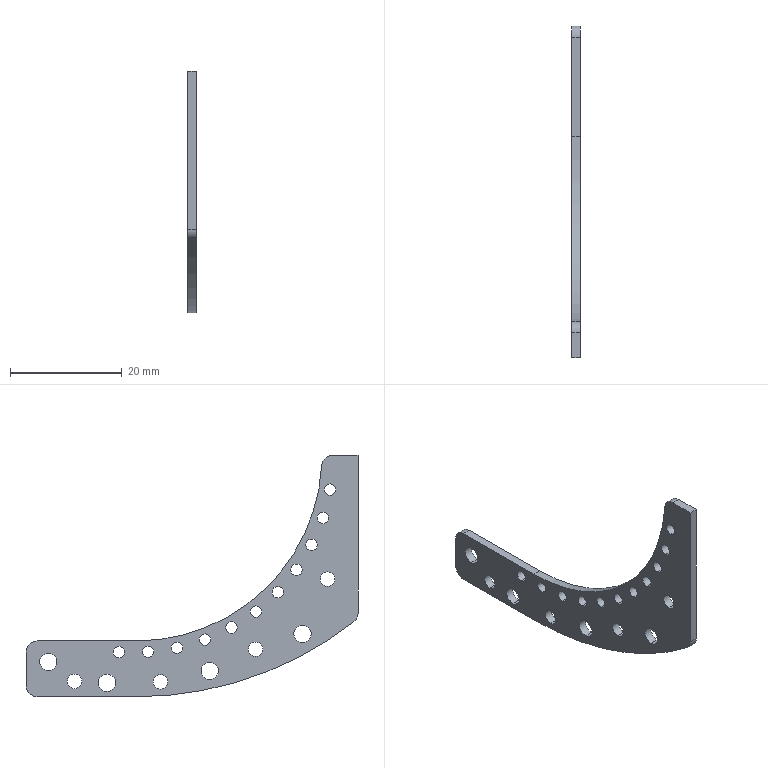Part | SolidWorks | features Extrusion 1, Fillet 1 | 1 solid | 51 faces | box 1.5 x 59.45 x 43.25 mm | volume 1169 mm3 | cylinder 44 | plane 7 | commonest cylinder face diameters 2.05 x22 2.6 x8 3.1 x8 4 x4 66.5 x1 126.5 x1